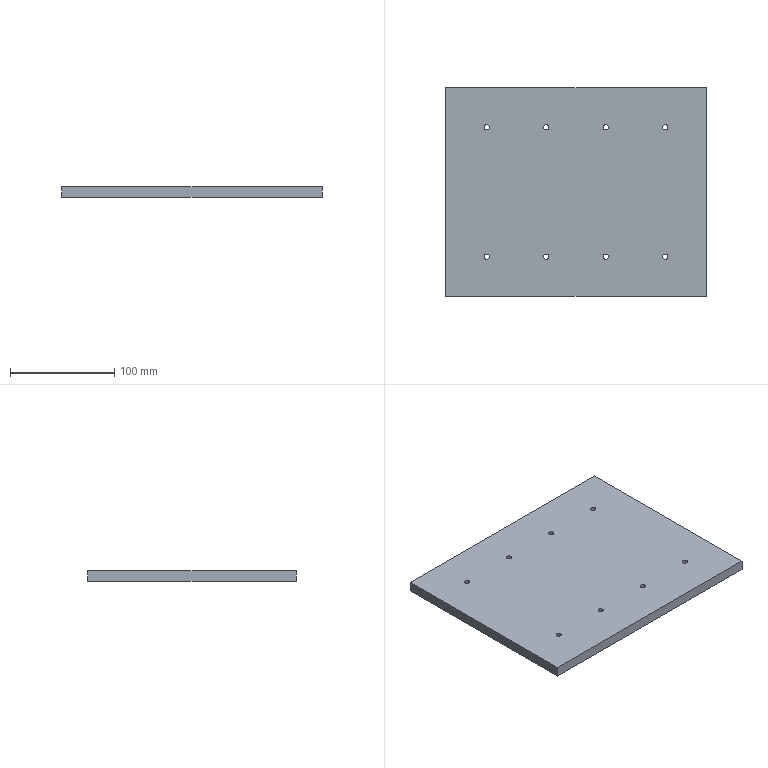Part | SolidWorks | features Extrusion 1, HoleWzd 1 | 1 solid | 22 faces | box 250 x 200 x 10 mm | volume 498429 mm3 | cylinder 16 | plane 6 | commonest cylinder face diameters 5 x16
STEP:
#1=CARTESIAN_POINT('',(-88.,62.,0.));
#2=VERTEX_POINT('',#1);
#3=CARTESIAN_POINT('',(-83.,62.,0.));
#4=VERTEX_POINT('',#3);
#5=CARTESIAN_POINT('',(-85.5,62.,0.));
#6=DIRECTION('',(0.,0.,1.));
#7=DIRECTION('',(1.,0.,0.));
#8=AXIS2_PLACEMENT_3D('',#5,#6,#7);
#9=CIRCLE('',#8,2.5);
#10=EDGE_CURVE('',#2,#4,#9,.T.);
#11=ORIENTED_EDGE('',*,*,#10,.F.);
#12=CARTESIAN_POINT('',(-88.,62.,10.));
#13=VERTEX_POINT('',#12);
#14=CARTESIAN_POINT('',(-88.,62.,10.));
#15=DIRECTION('',(0.,0.,1.));
#16=VECTOR('',#15,1000.);
#17=LINE('',#14,#16);
#18=EDGE_CURVE('',#2,#13,#17,.T.);
#19=ORIENTED_EDGE('',*,*,#18,.T.);
#20=CARTESIAN_POINT('',(-83.,62.,10.));
#21=VERTEX_POINT('',#20);
#22=CARTESIAN_POINT('',(-85.5,62.,10.));
#23=DIRECTION('',(0.,0.,1.));
#24=DIRECTION('',(1.,0.,0.));
#25=AXIS2_PLACEMENT_3D('',#22,#23,#24);
#26=CIRCLE('',#25,2.5);
#27=EDGE_CURVE('',#13,#21,#26,.T.);
#28=ORIENTED_EDGE('',*,*,#27,.T.);
#29=CARTESIAN_POINT('',(-83.,62.,10.));
#30=DIRECTION('',(0.,0.,1.));
#31=VECTOR('',#30,1000.);
#32=LINE('',#29,#31);
#33=EDGE_CURVE('',#4,#21,#32,.T.);
#34=ORIENTED_EDGE('',*,*,#33,.F.);
#35=EDGE_LOOP('',(#11,#19,#28,#34));
#36=FACE_OUTER_BOUND('',#35,.T.);
#37=CARTESIAN_POINT('',(-85.5,62.,10.));
#38=DIRECTION('',(0.,0.,1.));
#39=DIRECTION('',(1.,0.,0.));
#40=AXIS2_PLACEMENT_3D('',#37,#38,#39);
#41=CYLINDRICAL_SURFACE('',#40,2.5);
#42=ADVANCED_FACE('',(#36),#41,.F.);
#43=CARTESIAN_POINT('',(-31.,62.,0.));
#44=VERTEX_POINT('',#43);
#45=CARTESIAN_POINT('',(-26.,62.,0.));
#46=VERTEX_POINT('',#45);
#47=CARTESIAN_POINT('',(-28.5,62.,0.));
#48=DIRECTION('',(0.,0.,1.));
#49=DIRECTION('',(1.,0.,0.));
#50=AXIS2_PLACEMENT_3D('',#47,#48,#49);
#51=CIRCLE('',#50,2.5);
#52=EDGE_CURVE('',#44,#46,#51,.T.);
#53=ORIENTED_EDGE('',*,*,#52,.F.);
#54=CARTESIAN_POINT('',(-31.,62.,10.));
#55=VERTEX_POINT('',#54);
#56=CARTESIAN_POINT('',(-31.,62.,10.));
#57=DIRECTION('',(0.,0.,1.));
#58=VECTOR('',#57,1000.);
#59=LINE('',#56,#58);
#60=EDGE_CURVE('',#44,#55,#59,.T.);
#61=ORIENTED_EDGE('',*,*,#60,.T.);
#62=CARTESIAN_POINT('',(-26.,62.,10.));
#63=VERTEX_POINT('',#62);
#64=CARTESIAN_POINT('',(-28.5,62.,10.));
#65=DIRECTION('',(0.,0.,1.));
#66=DIRECTION('',(1.,0.,0.));
#67=AXIS2_PLACEMENT_3D('',#64,#65,#66);
#68=CIRCLE('',#67,2.5);
#69=EDGE_CURVE('',#55,#63,#68,.T.);
#70=ORIENTED_EDGE('',*,*,#69,.T.);
#71=CARTESIAN_POINT('',(-26.,62.,10.));
#72=DIRECTION('',(0.,0.,1.));
#73=VECTOR('',#72,1000.);
#74=LINE('',#71,#73);
#75=EDGE_CURVE('',#46,#63,#74,.T.);
#76=ORIENTED_EDGE('',*,*,#75,.F.);
#77=EDGE_LOOP('',(#53,#61,#70,#76));
#78=FACE_OUTER_BOUND('',#77,.T.);
#79=CARTESIAN_POINT('',(-28.5,62.,10.));
#80=DIRECTION('',(0.,0.,1.));
#81=DIRECTION('',(1.,0.,0.));
#82=AXIS2_PLACEMENT_3D('',#79,#80,#81);
#83=CYLINDRICAL_SURFACE('',#82,2.5);
#84=ADVANCED_FACE('',(#78),#83,.F.);
#85=CARTESIAN_POINT('',(83.,62.,0.));
#86=VERTEX_POINT('',#85);
#87=CARTESIAN_POINT('',(88.,62.,0.));
#88=VERTEX_POINT('',#87);
#89=CARTESIAN_POINT('',(85.5,62.,0.));
#90=DIRECTION('',(0.,0.,1.));
#91=DIRECTION('',(1.,0.,0.));
#92=AXIS2_PLACEMENT_3D('',#89,#90,#91);
#93=CIRCLE('',#92,2.5);
#94=EDGE_CURVE('',#86,#88,#93,.T.);
#95=ORIENTED_EDGE('',*,*,#94,.F.);
#96=CARTESIAN_POINT('',(83.,62.,10.));
#97=VERTEX_POINT('',#96);
#98=CARTESIAN_POINT('',(83.,62.,10.));
#99=DIRECTION('',(0.,0.,1.));
#100=VECTOR('',#99,1000.);
#101=LINE('',#98,#100);
#102=EDGE_CURVE('',#86,#97,#101,.T.);
#103=ORIENTED_EDGE('',*,*,#102,.T.);
#104=CARTESIAN_POINT('',(88.,62.,10.));
#105=VERTEX_POINT('',#104);
#106=CARTESIAN_POINT('',(85.5,62.,10.));
#107=DIRECTION('',(0.,0.,1.));
#108=DIRECTION('',(1.,0.,0.));
#109=AXIS2_PLACEMENT_3D('',#106,#107,#108);
#110=CIRCLE('',#109,2.5);
#111=EDGE_CURVE('',#97,#105,#110,.T.);
#112=ORIENTED_EDGE('',*,*,#111,.T.);
#113=CARTESIAN_POINT('',(88.,62.,10.));
#114=DIRECTION('',(0.,0.,1.));
#115=VECTOR('',#114,1000.);
#116=LINE('',#113,#115);
#117=EDGE_CURVE('',#88,#105,#116,.T.);
#118=ORIENTED_EDGE('',*,*,#117,.F.);
#119=EDGE_LOOP('',(#95,#103,#112,#118));
#120=FACE_OUTER_BOUND('',#119,.T.);
#121=CARTESIAN_POINT('',(85.5,62.,10.));
#122=DIRECTION('',(0.,0.,1.));
#123=DIRECTION('',(1.,0.,0.));
#124=AXIS2_PLACEMENT_3D('',#121,#122,#123);
#125=CYLINDRICAL_SURFACE('',#124,2.5);
#126=ADVANCED_FACE('',(#120),#125,.F.);
#127=CARTESIAN_POINT('',(26.,62.,0.));
#128=VERTEX_POINT('',#127);
#129=CARTESIAN_POINT('',(31.,62.,0.));
#130=VERTEX_POINT('',#129);
#131=CARTESIAN_POINT('',(28.5,62.,0.));
#132=DIRECTION('',(0.,0.,1.));
#133=DIRECTION('',(1.,0.,0.));
#134=AXIS2_PLACEMENT_3D('',#131,#132,#133);
#135=CIRCLE('',#134,2.5);
#136=EDGE_CURVE('',#128,#130,#135,.T.);
#137=ORIENTED_EDGE('',*,*,#136,.F.);
#138=CARTESIAN_POINT('',(26.,62.,10.));
#139=VERTEX_POINT('',#138);
#140=CARTESIAN_POINT('',(26.,62.,10.));
#141=DIRECTION('',(0.,0.,1.));
#142=VECTOR('',#141,1000.);
#143=LINE('',#140,#142);
#144=EDGE_CURVE('',#128,#139,#143,.T.);
#145=ORIENTED_EDGE('',*,*,#144,.T.);
#146=CARTESIAN_POINT('',(31.,62.,10.));
#147=VERTEX_POINT('',#146);
#148=CARTESIAN_POINT('',(28.5,62.,10.));
#149=DIRECTION('',(0.,0.,1.));
#150=DIRECTION('',(1.,0.,0.));
#151=AXIS2_PLACEMENT_3D('',#148,#149,#150);
#152=CIRCLE('',#151,2.5);
#153=EDGE_CURVE('',#139,#147,#152,.T.);
#154=ORIENTED_EDGE('',*,*,#153,.T.);
#155=CARTESIAN_POINT('',(31.,62.,10.));
#156=DIRECTION('',(0.,0.,1.));
#157=VECTOR('',#156,1000.);
#158=LINE('',#155,#157);
#159=EDGE_CURVE('',#130,#147,#158,.T.);
#160=ORIENTED_EDGE('',*,*,#159,.F.);
#161=EDGE_LOOP('',(#137,#145,#154,#160));
#162=FACE_OUTER_BOUND('',#161,.T.);
#163=CARTESIAN_POINT('',(28.5,62.,10.));
#164=DIRECTION('',(0.,0.,1.));
#165=DIRECTION('',(1.,0.,0.));
#166=AXIS2_PLACEMENT_3D('',#163,#164,#165);
#167=CYLINDRICAL_SURFACE('',#166,2.5);
#168=ADVANCED_FACE('',(#162),#167,.F.);
#169=CARTESIAN_POINT('',(26.,-62.,0.));
#170=VERTEX_POINT('',#169);
#171=CARTESIAN_POINT('',(31.,-62.,0.));
#172=VERTEX_POINT('',#171);
#173=CARTESIAN_POINT('',(28.5,-62.,0.));
#174=DIRECTION('',(0.,0.,1.));
#175=DIRECTION('',(1.,0.,0.));
#176=AXIS2_PLACEMENT_3D('',#173,#174,#175);
#177=CIRCLE('',#176,2.5);
#178=EDGE_CURVE('',#170,#172,#177,.T.);
#179=ORIENTED_EDGE('',*,*,#178,.F.);
#180=CARTESIAN_POINT('',(26.,-62.,10.));
#181=VERTEX_POINT('',#180);
#182=CARTESIAN_POINT('',(26.,-62.,10.));
#183=DIRECTION('',(0.,0.,1.));
#184=VECTOR('',#183,1000.);
#185=LINE('',#182,#184);
#186=EDGE_CURVE('',#170,#181,#185,.T.);
#187=ORIENTED_EDGE('',*,*,#186,.T.);
#188=CARTESIAN_POINT('',(31.,-62.,10.));
#189=VERTEX_POINT('',#188);
#190=CARTESIAN_POINT('',(28.5,-62.,10.));
#191=DIRECTION('',(0.,0.,1.));
#192=DIRECTION('',(1.,0.,0.));
#193=AXIS2_PLACEMENT_3D('',#190,#191,#192);
#194=CIRCLE('',#193,2.5);
#195=EDGE_CURVE('',#181,#189,#194,.T.);
#196=ORIENTED_EDGE('',*,*,#195,.T.);
#197=CARTESIAN_POINT('',(31.,-62.,10.));
#198=DIRECTION('',(0.,0.,1.));
#199=VECTOR('',#198,1000.);
#200=LINE('',#197,#199);
#201=EDGE_CURVE('',#172,#189,#200,.T.);
#202=ORIENTED_EDGE('',*,*,#201,.F.);
#203=EDGE_LOOP('',(#179,#187,#196,#202));
#204=FACE_OUTER_BOUND('',#203,.T.);
#205=CARTESIAN_POINT('',(28.5,-62.,10.));
#206=DIRECTION('',(0.,0.,1.));
#207=DIRECTION('',(1.,0.,0.));
#208=AXIS2_PLACEMENT_3D('',#205,#206,#207);
#209=CYLINDRICAL_SURFACE('',#208,2.5);
#210=ADVANCED_FACE('',(#204),#209,.F.);
#211=CARTESIAN_POINT('',(83.,-62.,0.));
#212=VERTEX_POINT('',#211);
#213=CARTESIAN_POINT('',(88.,-62.,0.));
#214=VERTEX_POINT('',#213);
#215=CARTESIAN_POINT('',(85.5,-62.,0.));
#216=DIRECTION('',(0.,0.,1.));
#217=DIRECTION('',(1.,0.,0.));
#218=AXIS2_PLACEMENT_3D('',#215,#216,#217);
#219=CIRCLE('',#218,2.5);
#220=EDGE_CURVE('',#212,#214,#219,.T.);
#221=ORIENTED_EDGE('',*,*,#220,.F.);
#222=CARTESIAN_POINT('',(83.,-62.,10.));
#223=VERTEX_POINT('',#222);
#224=CARTESIAN_POINT('',(83.,-62.,10.));
#225=DIRECTION('',(0.,0.,1.));
#226=VECTOR('',#225,1000.);
#227=LINE('',#224,#226);
#228=EDGE_CURVE('',#212,#223,#227,.T.);
#229=ORIENTED_EDGE('',*,*,#228,.T.);
#230=CARTESIAN_POINT('',(88.,-62.,10.));
#231=VERTEX_POINT('',#230);
#232=CARTESIAN_POINT('',(85.5,-62.,10.));
#233=DIRECTION('',(0.,0.,1.));
#234=DIRECTION('',(1.,0.,0.));
#235=AXIS2_PLACEMENT_3D('',#232,#233,#234);
#236=CIRCLE('',#235,2.5);
#237=EDGE_CURVE('',#223,#231,#236,.T.);
#238=ORIENTED_EDGE('',*,*,#237,.T.);
#239=CARTESIAN_POINT('',(88.,-62.,10.));
#240=DIRECTION('',(0.,0.,1.));
#241=VECTOR('',#240,1000.);
#242=LINE('',#239,#241);
#243=EDGE_CURVE('',#214,#231,#242,.T.);
#244=ORIENTED_EDGE('',*,*,#243,.F.);
#245=EDGE_LOOP('',(#221,#229,#238,#244));
#246=FACE_OUTER_BOUND('',#245,.T.);
#247=CARTESIAN_POINT('',(85.5,-62.,10.));
#248=DIRECTION('',(0.,0.,1.));
#249=DIRECTION('',(1.,0.,0.));
#250=AXIS2_PLACEMENT_3D('',#247,#248,#249);
#251=CYLINDRICAL_SURFACE('',#250,2.5);
#252=ADVANCED_FACE('',(#246),#251,.F.);
#253=CARTESIAN_POINT('',(-31.,-62.,0.));
#254=VERTEX_POINT('',#253);
#255=CARTESIAN_POINT('',(-26.,-62.,0.));
#256=VERTEX_POINT('',#255);
#257=CARTESIAN_POINT('',(-28.5,-62.,0.));
#258=DIRECTION('',(0.,0.,1.));
#259=DIRECTION('',(1.,0.,0.));
#260=AXIS2_PLACEMENT_3D('',#257,#258,#259);
#261=CIRCLE('',#260,2.5);
#262=EDGE_CURVE('',#254,#256,#261,.T.);
#263=ORIENTED_EDGE('',*,*,#262,.F.);
#264=CARTESIAN_POINT('',(-31.,-62.,10.));
#265=VERTEX_POINT('',#264);
#266=CARTESIAN_POINT('',(-31.,-62.,10.));
#267=DIRECTION('',(0.,0.,1.));
#268=VECTOR('',#267,1000.);
#269=LINE('',#266,#268);
#270=EDGE_CURVE('',#254,#265,#269,.T.);
#271=ORIENTED_EDGE('',*,*,#270,.T.);
#272=CARTESIAN_POINT('',(-26.,-62.,10.));
#273=VERTEX_POINT('',#272);
#274=CARTESIAN_POINT('',(-28.5,-62.,10.));
#275=DIRECTION('',(0.,0.,1.));
#276=DIRECTION('',(1.,0.,0.));
#277=AXIS2_PLACEMENT_3D('',#274,#275,#276);
#278=CIRCLE('',#277,2.5);
#279=EDGE_CURVE('',#265,#273,#278,.T.);
#280=ORIENTED_EDGE('',*,*,#279,.T.);
#281=CARTESIAN_POINT('',(-26.,-62.,10.));
#282=DIRECTION('',(0.,0.,1.));
#283=VECTOR('',#282,1000.);
#284=LINE('',#281,#283);
#285=EDGE_CURVE('',#256,#273,#284,.T.);
#286=ORIENTED_EDGE('',*,*,#285,.F.);
#287=EDGE_LOOP('',(#263,#271,#280,#286));
#288=FACE_OUTER_BOUND('',#287,.T.);
#289=CARTESIAN_POINT('',(-28.5,-62.,10.));
#290=DIRECTION('',(0.,0.,1.));
#291=DIRECTION('',(1.,0.,0.));
#292=AXIS2_PLACEMENT_3D('',#289,#290,#291);
#293=CYLINDRICAL_SURFACE('',#292,2.5);
#294=ADVANCED_FACE('',(#288),#293,.F.);
#295=CARTESIAN_POINT('',(-88.,-62.,0.));
#296=VERTEX_POINT('',#295);
#297=CARTESIAN_POINT('',(-83.,-62.,0.));
#298=VERTEX_POINT('',#297);
#299=CARTESIAN_POINT('',(-85.5,-62.,0.));
#300=DIRECTION('',(0.,0.,1.));
#301=DIRECTION('',(1.,0.,0.));
#302=AXIS2_PLACEMENT_3D('',#299,#300,#301);
#303=CIRCLE('',#302,2.5);
#304=EDGE_CURVE('',#296,#298,#303,.T.);
#305=ORIENTED_EDGE('',*,*,#304,.F.);
#306=CARTESIAN_POINT('',(-88.,-62.,10.));
#307=VERTEX_POINT('',#306);
#308=CARTESIAN_POINT('',(-88.,-62.,10.));
#309=DIRECTION('',(0.,0.,1.));
#310=VECTOR('',#309,1000.);
#311=LINE('',#308,#310);
#312=EDGE_CURVE('',#296,#307,#311,.T.);
#313=ORIENTED_EDGE('',*,*,#312,.T.);
#314=CARTESIAN_POINT('',(-83.,-62.,10.));
#315=VERTEX_POINT('',#314);
#316=CARTESIAN_POINT('',(-85.5,-62.,10.));
#317=DIRECTION('',(0.,0.,1.));
#318=DIRECTION('',(1.,0.,0.));
#319=AXIS2_PLACEMENT_3D('',#316,#317,#318);
#320=CIRCLE('',#319,2.5);
#321=EDGE_CURVE('',#307,#315,#320,.T.);
#322=ORIENTED_EDGE('',*,*,#321,.T.);
#323=CARTESIAN_POINT('',(-83.,-62.,10.));
#324=DIRECTION('',(0.,0.,1.));
#325=VECTOR('',#324,1000.);
#326=LINE('',#323,#325);
#327=EDGE_CURVE('',#298,#315,#326,.T.);
#328=ORIENTED_EDGE('',*,*,#327,.F.);
#329=EDGE_LOOP('',(#305,#313,#322,#328));
#330=FACE_OUTER_BOUND('',#329,.T.);
#331=CARTESIAN_POINT('',(-85.5,-62.,10.));
#332=DIRECTION('',(0.,0.,1.));
#333=DIRECTION('',(1.,0.,0.));
#334=AXIS2_PLACEMENT_3D('',#331,#332,#333);
#335=CYLINDRICAL_SURFACE('',#334,2.5);
#336=ADVANCED_FACE('',(#330),#335,.F.);
#337=CARTESIAN_POINT('',(125.,-100.,0.));
#338=VERTEX_POINT('',#337);
#339=CARTESIAN_POINT('',(125.,100.,0.));
#340=VERTEX_POINT('',#339);
#341=CARTESIAN_POINT('',(125.,100.,0.));
#342=DIRECTION('',(0.,1.,0.));
#343=VECTOR('',#342,1000.);
#344=LINE('',#341,#343);
#345=EDGE_CURVE('',#338,#340,#344,.T.);
#346=ORIENTED_EDGE('',*,*,#345,.T.);
#347=CARTESIAN_POINT('',(125.,100.,10.));
#348=VERTEX_POINT('',#347);
#349=CARTESIAN_POINT('',(125.,100.,10.));
#350=DIRECTION('',(0.,0.,-1.));
#351=VECTOR('',#350,1000.);
#352=LINE('',#349,#351);
#353=EDGE_CURVE('',#348,#340,#352,.T.);
#354=ORIENTED_EDGE('',*,*,#353,.F.);
#355=CARTESIAN_POINT('',(125.,-100.,10.));
#356=VERTEX_POINT('',#355);
#357=CARTESIAN_POINT('',(125.,100.,10.));
#358=DIRECTION('',(0.,1.,0.));
#359=VECTOR('',#358,1000.);
#360=LINE('',#357,#359);
#361=EDGE_CURVE('',#356,#348,#360,.T.);
#362=ORIENTED_EDGE('',*,*,#361,.F.);
#363=CARTESIAN_POINT('',(125.,-100.,10.));
#364=DIRECTION('',(0.,0.,-1.));
#365=VECTOR('',#364,1000.);
#366=LINE('',#363,#365);
#367=EDGE_CURVE('',#356,#338,#366,.T.);
#368=ORIENTED_EDGE('',*,*,#367,.T.);
#369=EDGE_LOOP('',(#346,#354,#362,#368));
#370=FACE_OUTER_BOUND('',#369,.T.);
#371=CARTESIAN_POINT('',(125.,100.,10.));
#372=DIRECTION('',(-1.,0.,0.));
#373=DIRECTION('',(0.,0.,1.));
#374=AXIS2_PLACEMENT_3D('',#371,#372,#373);
#375=PLANE('',#374);
#376=ADVANCED_FACE('',(#370),#375,.F.);
#377=CARTESIAN_POINT('',(-125.,100.,0.));
#378=VERTEX_POINT('',#377);
#379=CARTESIAN_POINT('',(-125.,100.,0.));
#380=DIRECTION('',(-1.,0.,0.));
#381=VECTOR('',#380,1000.);
#382=LINE('',#379,#381);
#383=EDGE_CURVE('',#340,#378,#382,.T.);
#384=ORIENTED_EDGE('',*,*,#383,.T.);
#385=CARTESIAN_POINT('',(-125.,100.,10.));
#386=VERTEX_POINT('',#385);
#387=CARTESIAN_POINT('',(-125.,100.,10.));
#388=DIRECTION('',(0.,0.,-1.));
#389=VECTOR('',#388,1000.);
#390=LINE('',#387,#389);
#391=EDGE_CURVE('',#386,#378,#390,.T.);
#392=ORIENTED_EDGE('',*,*,#391,.F.);
#393=CARTESIAN_POINT('',(-125.,100.,10.));
#394=DIRECTION('',(-1.,0.,0.));
#395=VECTOR('',#394,1000.);
#396=LINE('',#393,#395);
#397=EDGE_CURVE('',#348,#386,#396,.T.);
#398=ORIENTED_EDGE('',*,*,#397,.F.);
#399=ORIENTED_EDGE('',*,*,#353,.T.);
#400=EDGE_LOOP('',(#384,#392,#398,#399));
#401=FACE_OUTER_BOUND('',#400,.T.);
#402=CARTESIAN_POINT('',(-125.,100.,10.));
#403=DIRECTION('',(0.,-1.,0.));
#404=DIRECTION('',(0.,0.,-1.));
#405=AXIS2_PLACEMENT_3D('',#402,#403,#404);
#406=PLANE('',#405);
#407=ADVANCED_FACE('',(#401),#406,.F.);
#408=CARTESIAN_POINT('',(-125.,-100.,0.));
#409=VERTEX_POINT('',#408);
#410=CARTESIAN_POINT('',(-125.,100.,0.));
#411=DIRECTION('',(0.,-1.,0.));
#412=VECTOR('',#411,1000.);
#413=LINE('',#410,#412);
#414=EDGE_CURVE('',#378,#409,#413,.T.);
#415=ORIENTED_EDGE('',*,*,#414,.T.);
#416=CARTESIAN_POINT('',(-125.,-100.,10.));
#417=VERTEX_POINT('',#416);
#418=CARTESIAN_POINT('',(-125.,-100.,10.));
#419=DIRECTION('',(0.,0.,-1.));
#420=VECTOR('',#419,1000.);
#421=LINE('',#418,#420);
#422=EDGE_CURVE('',#417,#409,#421,.T.);
#423=ORIENTED_EDGE('',*,*,#422,.F.);
#424=CARTESIAN_POINT('',(-125.,100.,10.));
#425=DIRECTION('',(0.,-1.,0.));
#426=VECTOR('',#425,1000.);
#427=LINE('',#424,#426);
#428=EDGE_CURVE('',#386,#417,#427,.T.);
#429=ORIENTED_EDGE('',*,*,#428,.F.);
#430=ORIENTED_EDGE('',*,*,#391,.T.);
#431=EDGE_LOOP('',(#415,#423,#429,#430));
#432=FACE_OUTER_BOUND('',#431,.T.);
#433=CARTESIAN_POINT('',(-125.,100.,10.));
#434=DIRECTION('',(1.,0.,0.));
#435=DIRECTION('',(0.,1.,0.));
#436=AXIS2_PLACEMENT_3D('',#433,#434,#435);
#437=PLANE('',#436);
#438=ADVANCED_FACE('',(#432),#437,.F.);
#439=CARTESIAN_POINT('',(-125.,-100.,0.));
#440=DIRECTION('',(1.,0.,0.));
#441=VECTOR('',#440,1000.);
#442=LINE('',#439,#441);
#443=EDGE_CURVE('',#409,#338,#442,.T.);
#444=ORIENTED_EDGE('',*,*,#443,.T.);
#445=ORIENTED_EDGE('',*,*,#367,.F.);
#446=CARTESIAN_POINT('',(-125.,-100.,10.));
#447=DIRECTION('',(1.,0.,0.));
#448=VECTOR('',#447,1000.);
#449=LINE('',#446,#448);
#450=EDGE_CURVE('',#417,#356,#449,.T.);
#451=ORIENTED_EDGE('',*,*,#450,.F.);
#452=ORIENTED_EDGE('',*,*,#422,.T.);
#453=EDGE_LOOP('',(#444,#445,#451,#452));
#454=FACE_OUTER_BOUND('',#453,.T.);
#455=CARTESIAN_POINT('',(-125.,-100.,10.));
#456=DIRECTION('',(0.,1.,0.));
#457=DIRECTION('',(0.,0.,1.));
#458=AXIS2_PLACEMENT_3D('',#455,#456,#457);
#459=PLANE('',#458);
#460=ADVANCED_FACE('',(#454),#459,.F.);
#461=CARTESIAN_POINT('',(-85.5,62.,10.));
#462=DIRECTION('',(0.,0.,1.));
#463=DIRECTION('',(1.,0.,0.));
#464=AXIS2_PLACEMENT_3D('',#461,#462,#463);
#465=CIRCLE('',#464,2.5);
#466=EDGE_CURVE('',#21,#13,#465,.T.);
#467=ORIENTED_EDGE('',*,*,#466,.F.);
#468=ORIENTED_EDGE('',*,*,#27,.F.);
#469=EDGE_LOOP('',(#467,#468));
#470=FACE_BOUND('',#469,.T.);
#471=CARTESIAN_POINT('',(-28.5,62.,10.));
#472=DIRECTION('',(0.,0.,1.));
#473=DIRECTION('',(1.,0.,0.));
#474=AXIS2_PLACEMENT_3D('',#471,#472,#473);
#475=CIRCLE('',#474,2.5);
#476=EDGE_CURVE('',#63,#55,#475,.T.);
#477=ORIENTED_EDGE('',*,*,#476,.F.);
#478=ORIENTED_EDGE('',*,*,#69,.F.);
#479=EDGE_LOOP('',(#477,#478));
#480=FACE_BOUND('',#479,.T.);
#481=CARTESIAN_POINT('',(85.5,62.,10.));
#482=DIRECTION('',(0.,0.,1.));
#483=DIRECTION('',(1.,0.,0.));
#484=AXIS2_PLACEMENT_3D('',#481,#482,#483);
#485=CIRCLE('',#484,2.5);
#486=EDGE_CURVE('',#105,#97,#485,.T.);
#487=ORIENTED_EDGE('',*,*,#486,.F.);
#488=ORIENTED_EDGE('',*,*,#111,.F.);
#489=EDGE_LOOP('',(#487,#488));
#490=FACE_BOUND('',#489,.T.);
#491=CARTESIAN_POINT('',(28.5,62.,10.));
#492=DIRECTION('',(0.,0.,1.));
#493=DIRECTION('',(1.,0.,0.));
#494=AXIS2_PLACEMENT_3D('',#491,#492,#493);
#495=CIRCLE('',#494,2.5);
#496=EDGE_CURVE('',#147,#139,#495,.T.);
#497=ORIENTED_EDGE('',*,*,#496,.F.);
#498=ORIENTED_EDGE('',*,*,#153,.F.);
#499=EDGE_LOOP('',(#497,#498));
#500=FACE_BOUND('',#499,.T.);
#501=CARTESIAN_POINT('',(28.5,-62.,10.));
#502=DIRECTION('',(0.,0.,1.));
#503=DIRECTION('',(1.,0.,0.));
#504=AXIS2_PLACEMENT_3D('',#501,#502,#503);
#505=CIRCLE('',#504,2.5);
#506=EDGE_CURVE('',#189,#181,#505,.T.);
#507=ORIENTED_EDGE('',*,*,#506,.F.);
#508=ORIENTED_EDGE('',*,*,#195,.F.);
#509=EDGE_LOOP('',(#507,#508));
#510=FACE_BOUND('',#509,.T.);
#511=CARTESIAN_POINT('',(85.5,-62.,10.));
#512=DIRECTION('',(0.,0.,1.));
#513=DIRECTION('',(1.,0.,0.));
#514=AXIS2_PLACEMENT_3D('',#511,#512,#513);
#515=CIRCLE('',#514,2.5);
#516=EDGE_CURVE('',#231,#223,#515,.T.);
#517=ORIENTED_EDGE('',*,*,#516,.F.);
#518=ORIENTED_EDGE('',*,*,#237,.F.);
#519=EDGE_LOOP('',(#517,#518));
#520=FACE_BOUND('',#519,.T.);
#521=CARTESIAN_POINT('',(-28.5,-62.,10.));
#522=DIRECTION('',(0.,0.,1.));
#523=DIRECTION('',(1.,0.,0.));
#524=AXIS2_PLACEMENT_3D('',#521,#522,#523);
#525=CIRCLE('',#524,2.5);
#526=EDGE_CURVE('',#273,#265,#525,.T.);
#527=ORIENTED_EDGE('',*,*,#526,.F.);
#528=ORIENTED_EDGE('',*,*,#279,.F.);
#529=EDGE_LOOP('',(#527,#528));
#530=FACE_BOUND('',#529,.T.);
#531=CARTESIAN_POINT('',(-85.5,-62.,10.));
#532=DIRECTION('',(0.,0.,1.));
#533=DIRECTION('',(1.,0.,0.));
#534=AXIS2_PLACEMENT_3D('',#531,#532,#533);
#535=CIRCLE('',#534,2.5);
#536=EDGE_CURVE('',#315,#307,#535,.T.);
#537=ORIENTED_EDGE('',*,*,#536,.F.);
#538=ORIENTED_EDGE('',*,*,#321,.F.);
#539=EDGE_LOOP('',(#537,#538));
#540=FACE_BOUND('',#539,.T.);
#541=ORIENTED_EDGE('',*,*,#361,.T.);
#542=ORIENTED_EDGE('',*,*,#397,.T.);
#543=ORIENTED_EDGE('',*,*,#428,.T.);
#544=ORIENTED_EDGE('',*,*,#450,.T.);
#545=EDGE_LOOP('',(#541,#542,#543,#544));
#546=FACE_OUTER_BOUND('',#545,.T.);
#547=CARTESIAN_POINT('',(0.,0.,10.));
#548=DIRECTION('',(0.,0.,1.));
#549=DIRECTION('',(1.,0.,0.));
#550=AXIS2_PLACEMENT_3D('',#547,#548,#549);
#551=PLANE('',#550);
#552=ADVANCED_FACE('',(#470,#480,#490,#500,#510,#520,#530,#540,#546),#551,.T.);
#553=CARTESIAN_POINT('',(-85.5,62.,0.));
#554=DIRECTION('',(0.,0.,1.));
#555=DIRECTION('',(1.,0.,0.));
#556=AXIS2_PLACEMENT_3D('',#553,#554,#555);
#557=CIRCLE('',#556,2.5);
#558=EDGE_CURVE('',#4,#2,#557,.T.);
#559=ORIENTED_EDGE('',*,*,#558,.T.);
#560=ORIENTED_EDGE('',*,*,#10,.T.);
#561=EDGE_LOOP('',(#559,#560));
#562=FACE_BOUND('',#561,.T.);
#563=CARTESIAN_POINT('',(-28.5,62.,0.));
#564=DIRECTION('',(0.,0.,1.));
#565=DIRECTION('',(1.,0.,0.));
#566=AXIS2_PLACEMENT_3D('',#563,#564,#565);
#567=CIRCLE('',#566,2.5);
#568=EDGE_CURVE('',#46,#44,#567,.T.);
#569=ORIENTED_EDGE('',*,*,#568,.T.);
#570=ORIENTED_EDGE('',*,*,#52,.T.);
#571=EDGE_LOOP('',(#569,#570));
#572=FACE_BOUND('',#571,.T.);
#573=CARTESIAN_POINT('',(85.5,62.,0.));
#574=DIRECTION('',(0.,0.,1.));
#575=DIRECTION('',(1.,0.,0.));
#576=AXIS2_PLACEMENT_3D('',#573,#574,#575);
#577=CIRCLE('',#576,2.5);
#578=EDGE_CURVE('',#88,#86,#577,.T.);
#579=ORIENTED_EDGE('',*,*,#578,.T.);
#580=ORIENTED_EDGE('',*,*,#94,.T.);
#581=EDGE_LOOP('',(#579,#580));
#582=FACE_BOUND('',#581,.T.);
#583=CARTESIAN_POINT('',(28.5,62.,0.));
#584=DIRECTION('',(0.,0.,1.));
#585=DIRECTION('',(1.,0.,0.));
#586=AXIS2_PLACEMENT_3D('',#583,#584,#585);
#587=CIRCLE('',#586,2.5);
#588=EDGE_CURVE('',#130,#128,#587,.T.);
#589=ORIENTED_EDGE('',*,*,#588,.T.);
#590=ORIENTED_EDGE('',*,*,#136,.T.);
#591=EDGE_LOOP('',(#589,#590));
#592=FACE_BOUND('',#591,.T.);
#593=CARTESIAN_POINT('',(28.5,-62.,0.));
#594=DIRECTION('',(0.,0.,1.));
#595=DIRECTION('',(1.,0.,0.));
#596=AXIS2_PLACEMENT_3D('',#593,#594,#595);
#597=CIRCLE('',#596,2.5);
#598=EDGE_CURVE('',#172,#170,#597,.T.);
#599=ORIENTED_EDGE('',*,*,#598,.T.);
#600=ORIENTED_EDGE('',*,*,#178,.T.);
#601=EDGE_LOOP('',(#599,#600));
#602=FACE_BOUND('',#601,.T.);
#603=CARTESIAN_POINT('',(85.5,-62.,0.));
#604=DIRECTION('',(0.,0.,1.));
#605=DIRECTION('',(1.,0.,0.));
#606=AXIS2_PLACEMENT_3D('',#603,#604,#605);
#607=CIRCLE('',#606,2.5);
#608=EDGE_CURVE('',#214,#212,#607,.T.);
#609=ORIENTED_EDGE('',*,*,#608,.T.);
#610=ORIENTED_EDGE('',*,*,#220,.T.);
#611=EDGE_LOOP('',(#609,#610));
#612=FACE_BOUND('',#611,.T.);
#613=CARTESIAN_POINT('',(-28.5,-62.,0.));
#614=DIRECTION('',(0.,0.,1.));
#615=DIRECTION('',(1.,0.,0.));
#616=AXIS2_PLACEMENT_3D('',#613,#614,#615);
#617=CIRCLE('',#616,2.5);
#618=EDGE_CURVE('',#256,#254,#617,.T.);
#619=ORIENTED_EDGE('',*,*,#618,.T.);
#620=ORIENTED_EDGE('',*,*,#262,.T.);
#621=EDGE_LOOP('',(#619,#620));
#622=FACE_BOUND('',#621,.T.);
#623=CARTESIAN_POINT('',(-85.5,-62.,0.));
#624=DIRECTION('',(0.,0.,1.));
#625=DIRECTION('',(1.,0.,0.));
#626=AXIS2_PLACEMENT_3D('',#623,#624,#625);
#627=CIRCLE('',#626,2.5);
#628=EDGE_CURVE('',#298,#296,#627,.T.);
#629=ORIENTED_EDGE('',*,*,#628,.T.);
#630=ORIENTED_EDGE('',*,*,#304,.T.);
#631=EDGE_LOOP('',(#629,#630));
#632=FACE_BOUND('',#631,.T.);
#633=ORIENTED_EDGE('',*,*,#345,.F.);
#634=ORIENTED_EDGE('',*,*,#443,.F.);
#635=ORIENTED_EDGE('',*,*,#414,.F.);
#636=ORIENTED_EDGE('',*,*,#383,.F.);
#637=EDGE_LOOP('',(#633,#634,#635,#636));
#638=FACE_OUTER_BOUND('',#637,.T.);
#639=CARTESIAN_POINT('',(0.,0.,0.));
#640=DIRECTION('',(0.,0.,1.));
#641=DIRECTION('',(1.,0.,0.));
#642=AXIS2_PLACEMENT_3D('',#639,#640,#641);
#643=PLANE('',#642);
#644=ADVANCED_FACE('',(#562,#572,#582,#592,#602,#612,#622,#632,#638),#643,.F.);
#645=ORIENTED_EDGE('',*,*,#312,.F.);
#646=ORIENTED_EDGE('',*,*,#628,.F.);
#647=ORIENTED_EDGE('',*,*,#327,.T.);
#648=ORIENTED_EDGE('',*,*,#536,.T.);
#649=EDGE_LOOP('',(#645,#646,#647,#648));
#650=FACE_OUTER_BOUND('',#649,.T.);
#651=CARTESIAN_POINT('',(-85.5,-62.,10.));
#652=DIRECTION('',(0.,0.,1.));
#653=DIRECTION('',(1.,0.,0.));
#654=AXIS2_PLACEMENT_3D('',#651,#652,#653);
#655=CYLINDRICAL_SURFACE('',#654,2.5);
#656=ADVANCED_FACE('',(#650),#655,.F.);
#657=ORIENTED_EDGE('',*,*,#270,.F.);
#658=ORIENTED_EDGE('',*,*,#618,.F.);
#659=ORIENTED_EDGE('',*,*,#285,.T.);
#660=ORIENTED_EDGE('',*,*,#526,.T.);
#661=EDGE_LOOP('',(#657,#658,#659,#660));
#662=FACE_OUTER_BOUND('',#661,.T.);
#663=CARTESIAN_POINT('',(-28.5,-62.,10.));
#664=DIRECTION('',(0.,0.,1.));
#665=DIRECTION('',(1.,0.,0.));
#666=AXIS2_PLACEMENT_3D('',#663,#664,#665);
#667=CYLINDRICAL_SURFACE('',#666,2.5);
#668=ADVANCED_FACE('',(#662),#667,.F.);
#669=ORIENTED_EDGE('',*,*,#228,.F.);
#670=ORIENTED_EDGE('',*,*,#608,.F.);
#671=ORIENTED_EDGE('',*,*,#243,.T.);
#672=ORIENTED_EDGE('',*,*,#516,.T.);
#673=EDGE_LOOP('',(#669,#670,#671,#672));
#674=FACE_OUTER_BOUND('',#673,.T.);
#675=CARTESIAN_POINT('',(85.5,-62.,10.));
#676=DIRECTION('',(0.,0.,1.));
#677=DIRECTION('',(1.,0.,0.));
#678=AXIS2_PLACEMENT_3D('',#675,#676,#677);
#679=CYLINDRICAL_SURFACE('',#678,2.5);
#680=ADVANCED_FACE('',(#674),#679,.F.);
#681=ORIENTED_EDGE('',*,*,#186,.F.);
#682=ORIENTED_EDGE('',*,*,#598,.F.);
#683=ORIENTED_EDGE('',*,*,#201,.T.);
#684=ORIENTED_EDGE('',*,*,#506,.T.);
#685=EDGE_LOOP('',(#681,#682,#683,#684));
#686=FACE_OUTER_BOUND('',#685,.T.);
#687=CARTESIAN_POINT('',(28.5,-62.,10.));
#688=DIRECTION('',(0.,0.,1.));
#689=DIRECTION('',(1.,0.,0.));
#690=AXIS2_PLACEMENT_3D('',#687,#688,#689);
#691=CYLINDRICAL_SURFACE('',#690,2.5);
#692=ADVANCED_FACE('',(#686),#691,.F.);
#693=ORIENTED_EDGE('',*,*,#144,.F.);
#694=ORIENTED_EDGE('',*,*,#588,.F.);
#695=ORIENTED_EDGE('',*,*,#159,.T.);
#696=ORIENTED_EDGE('',*,*,#496,.T.);
#697=EDGE_LOOP('',(#693,#694,#695,#696));
#698=FACE_OUTER_BOUND('',#697,.T.);
#699=CARTESIAN_POINT('',(28.5,62.,10.));
#700=DIRECTION('',(0.,0.,1.));
#701=DIRECTION('',(1.,0.,0.));
#702=AXIS2_PLACEMENT_3D('',#699,#700,#701);
#703=CYLINDRICAL_SURFACE('',#702,2.5);
#704=ADVANCED_FACE('',(#698),#703,.F.);
#705=ORIENTED_EDGE('',*,*,#102,.F.);
#706=ORIENTED_EDGE('',*,*,#578,.F.);
#707=ORIENTED_EDGE('',*,*,#117,.T.);
#708=ORIENTED_EDGE('',*,*,#486,.T.);
#709=EDGE_LOOP('',(#705,#706,#707,#708));
#710=FACE_OUTER_BOUND('',#709,.T.);
#711=CARTESIAN_POINT('',(85.5,62.,10.));
#712=DIRECTION('',(0.,0.,1.));
#713=DIRECTION('',(1.,0.,0.));
#714=AXIS2_PLACEMENT_3D('',#711,#712,#713);
#715=CYLINDRICAL_SURFACE('',#714,2.5);
#716=ADVANCED_FACE('',(#710),#715,.F.);
#717=ORIENTED_EDGE('',*,*,#60,.F.);
#718=ORIENTED_EDGE('',*,*,#568,.F.);
#719=ORIENTED_EDGE('',*,*,#75,.T.);
#720=ORIENTED_EDGE('',*,*,#476,.T.);
#721=EDGE_LOOP('',(#717,#718,#719,#720));
#722=FACE_OUTER_BOUND('',#721,.T.);
#723=CARTESIAN_POINT('',(-28.5,62.,10.));
#724=DIRECTION('',(0.,0.,1.));
#725=DIRECTION('',(1.,0.,0.));
#726=AXIS2_PLACEMENT_3D('',#723,#724,#725);
#727=CYLINDRICAL_SURFACE('',#726,2.5);
#728=ADVANCED_FACE('',(#722),#727,.F.);
#729=ORIENTED_EDGE('',*,*,#18,.F.);
#730=ORIENTED_EDGE('',*,*,#558,.F.);
#731=ORIENTED_EDGE('',*,*,#33,.T.);
#732=ORIENTED_EDGE('',*,*,#466,.T.);
#733=EDGE_LOOP('',(#729,#730,#731,#732));
#734=FACE_OUTER_BOUND('',#733,.T.);
#735=CARTESIAN_POINT('',(-85.5,62.,10.));
#736=DIRECTION('',(0.,0.,1.));
#737=DIRECTION('',(1.,0.,0.));
#738=AXIS2_PLACEMENT_3D('',#735,#736,#737);
#739=CYLINDRICAL_SURFACE('',#738,2.5);
#740=ADVANCED_FACE('',(#734),#739,.F.);
#741=CLOSED_SHELL('',(#42,#84,#126,#168,#210,#252,#294,#336,#376,#407,#438,#460,#552,#644,#656,#668,#680,#692,#704,#716,#728,#740));
#742=MANIFOLD_SOLID_BREP('',#741);
#743=CARTESIAN_POINT('',(0.,0.,0.));
#744=DIRECTION('',(0.,0.,1.));
#745=DIRECTION('',(1.,0.,0.));
#746=AXIS2_PLACEMENT_3D('',#743,#744,#745);
#747=(LENGTH_UNIT()NAMED_UNIT(*)SI_UNIT(.MILLI.,.METRE.));
#748=UNCERTAINTY_MEASURE_WITH_UNIT(LENGTH_MEASURE(0.00001),#747,'','');
#749=(NAMED_UNIT(*)PLANE_ANGLE_UNIT()SI_UNIT($,.RADIAN.));
#750=(NAMED_UNIT(*)SI_UNIT($,.STERADIAN.)SOLID_ANGLE_UNIT());
#751=(GEOMETRIC_REPRESENTATION_CONTEXT(3)GLOBAL_UNCERTAINTY_ASSIGNED_CONTEXT((#748))GLOBAL_UNIT_ASSIGNED_CONTEXT((#747,#749,#750))REPRESENTATION_CONTEXT('',''));
#752=ADVANCED_BREP_SHAPE_REPRESENTATION('',(#742,#746),#751);